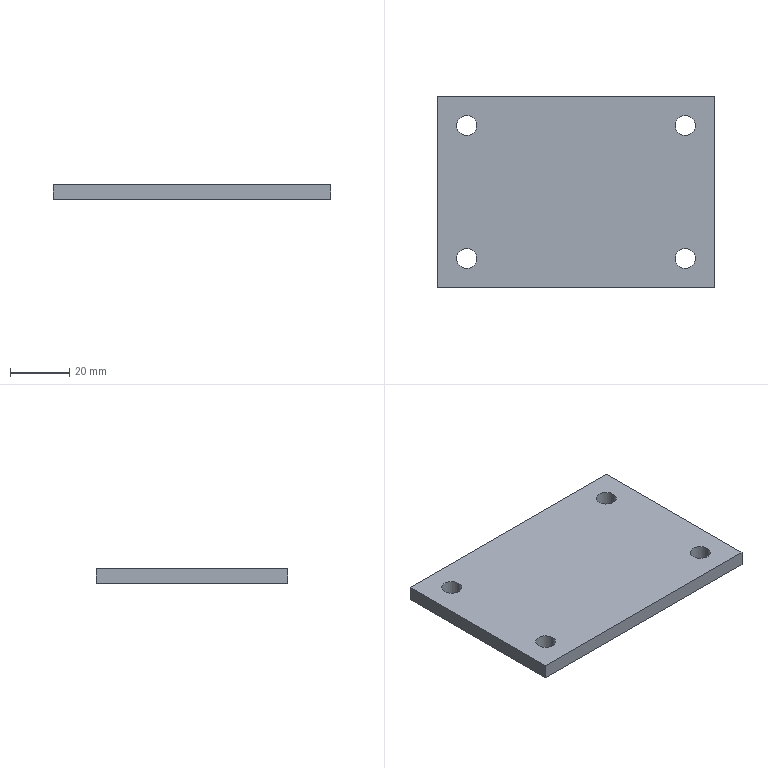Part | SolidWorks | features FlatPattern 1, SMBaseFlange 1, SheetMetal 1 | 1 solid | 14 faces | box 94 x 65 x 5 mm | volume 29824 mm3 | cylinder 8 | plane 6 | commonest cylinder face diameters 6.8 x8
STEP:
#1=CARTESIAN_POINT('',(-40.4,22.5,-5.));
#2=VERTEX_POINT('',#1);
#3=CARTESIAN_POINT('',(-33.6,22.5,-5.));
#4=VERTEX_POINT('',#3);
#5=CARTESIAN_POINT('',(-37.,22.5,-5.));
#6=DIRECTION('',(0.,0.,1.));
#7=DIRECTION('',(-1.,0.,0.));
#8=AXIS2_PLACEMENT_3D('',#5,#6,#7);
#9=CIRCLE('',#8,3.4);
#10=EDGE_CURVE('',#2,#4,#9,.T.);
#11=ORIENTED_EDGE('',*,*,#10,.F.);
#12=CARTESIAN_POINT('',(-40.4,22.5,0.));
#13=VERTEX_POINT('',#12);
#14=CARTESIAN_POINT('',(-40.4,22.5,-5.));
#15=DIRECTION('',(0.,0.,1.));
#16=VECTOR('',#15,1000.);
#17=LINE('',#14,#16);
#18=EDGE_CURVE('',#2,#13,#17,.T.);
#19=ORIENTED_EDGE('',*,*,#18,.T.);
#20=CARTESIAN_POINT('',(-33.6,22.5,0.));
#21=VERTEX_POINT('',#20);
#22=CARTESIAN_POINT('',(-37.,22.5,0.));
#23=DIRECTION('',(0.,0.,1.));
#24=DIRECTION('',(-1.,0.,0.));
#25=AXIS2_PLACEMENT_3D('',#22,#23,#24);
#26=CIRCLE('',#25,3.4);
#27=EDGE_CURVE('',#13,#21,#26,.T.);
#28=ORIENTED_EDGE('',*,*,#27,.T.);
#29=CARTESIAN_POINT('',(-33.6,22.5,-5.));
#30=DIRECTION('',(0.,0.,1.));
#31=VECTOR('',#30,1000.);
#32=LINE('',#29,#31);
#33=EDGE_CURVE('',#4,#21,#32,.T.);
#34=ORIENTED_EDGE('',*,*,#33,.F.);
#35=EDGE_LOOP('',(#11,#19,#28,#34));
#36=FACE_OUTER_BOUND('',#35,.T.);
#37=CARTESIAN_POINT('',(-37.,22.5,-5.));
#38=DIRECTION('',(0.,0.,1.));
#39=DIRECTION('',(1.,0.,0.));
#40=AXIS2_PLACEMENT_3D('',#37,#38,#39);
#41=CYLINDRICAL_SURFACE('',#40,3.4);
#42=ADVANCED_FACE('',(#36),#41,.F.);
#43=CARTESIAN_POINT('',(33.6,22.5,-5.));
#44=VERTEX_POINT('',#43);
#45=CARTESIAN_POINT('',(40.4,22.5,-5.));
#46=VERTEX_POINT('',#45);
#47=CARTESIAN_POINT('',(37.,22.5,-5.));
#48=DIRECTION('',(0.,0.,1.));
#49=DIRECTION('',(-1.,0.,0.));
#50=AXIS2_PLACEMENT_3D('',#47,#48,#49);
#51=CIRCLE('',#50,3.4);
#52=EDGE_CURVE('',#44,#46,#51,.T.);
#53=ORIENTED_EDGE('',*,*,#52,.F.);
#54=CARTESIAN_POINT('',(33.6,22.5,0.));
#55=VERTEX_POINT('',#54);
#56=CARTESIAN_POINT('',(33.6,22.5,-5.));
#57=DIRECTION('',(0.,0.,1.));
#58=VECTOR('',#57,1000.);
#59=LINE('',#56,#58);
#60=EDGE_CURVE('',#44,#55,#59,.T.);
#61=ORIENTED_EDGE('',*,*,#60,.T.);
#62=CARTESIAN_POINT('',(40.4,22.5,0.));
#63=VERTEX_POINT('',#62);
#64=CARTESIAN_POINT('',(37.,22.5,0.));
#65=DIRECTION('',(0.,0.,1.));
#66=DIRECTION('',(-1.,0.,0.));
#67=AXIS2_PLACEMENT_3D('',#64,#65,#66);
#68=CIRCLE('',#67,3.4);
#69=EDGE_CURVE('',#55,#63,#68,.T.);
#70=ORIENTED_EDGE('',*,*,#69,.T.);
#71=CARTESIAN_POINT('',(40.4,22.5,-5.));
#72=DIRECTION('',(0.,0.,1.));
#73=VECTOR('',#72,1000.);
#74=LINE('',#71,#73);
#75=EDGE_CURVE('',#46,#63,#74,.T.);
#76=ORIENTED_EDGE('',*,*,#75,.F.);
#77=EDGE_LOOP('',(#53,#61,#70,#76));
#78=FACE_OUTER_BOUND('',#77,.T.);
#79=CARTESIAN_POINT('',(37.,22.5,-5.));
#80=DIRECTION('',(0.,0.,1.));
#81=DIRECTION('',(1.,0.,0.));
#82=AXIS2_PLACEMENT_3D('',#79,#80,#81);
#83=CYLINDRICAL_SURFACE('',#82,3.4);
#84=ADVANCED_FACE('',(#78),#83,.F.);
#85=CARTESIAN_POINT('',(33.6,-22.5,-5.));
#86=VERTEX_POINT('',#85);
#87=CARTESIAN_POINT('',(40.4,-22.5,-5.));
#88=VERTEX_POINT('',#87);
#89=CARTESIAN_POINT('',(37.,-22.5,-5.));
#90=DIRECTION('',(0.,0.,1.));
#91=DIRECTION('',(1.,0.,0.));
#92=AXIS2_PLACEMENT_3D('',#89,#90,#91);
#93=CIRCLE('',#92,3.4);
#94=EDGE_CURVE('',#86,#88,#93,.T.);
#95=ORIENTED_EDGE('',*,*,#94,.F.);
#96=CARTESIAN_POINT('',(33.6,-22.5,0.));
#97=VERTEX_POINT('',#96);
#98=CARTESIAN_POINT('',(33.6,-22.5,-5.));
#99=DIRECTION('',(0.,0.,1.));
#100=VECTOR('',#99,1000.);
#101=LINE('',#98,#100);
#102=EDGE_CURVE('',#86,#97,#101,.T.);
#103=ORIENTED_EDGE('',*,*,#102,.T.);
#104=CARTESIAN_POINT('',(40.4,-22.5,0.));
#105=VERTEX_POINT('',#104);
#106=CARTESIAN_POINT('',(37.,-22.5,0.));
#107=DIRECTION('',(0.,0.,1.));
#108=DIRECTION('',(1.,0.,0.));
#109=AXIS2_PLACEMENT_3D('',#106,#107,#108);
#110=CIRCLE('',#109,3.4);
#111=EDGE_CURVE('',#97,#105,#110,.T.);
#112=ORIENTED_EDGE('',*,*,#111,.T.);
#113=CARTESIAN_POINT('',(40.4,-22.5,-5.));
#114=DIRECTION('',(0.,0.,1.));
#115=VECTOR('',#114,1000.);
#116=LINE('',#113,#115);
#117=EDGE_CURVE('',#88,#105,#116,.T.);
#118=ORIENTED_EDGE('',*,*,#117,.F.);
#119=EDGE_LOOP('',(#95,#103,#112,#118));
#120=FACE_OUTER_BOUND('',#119,.T.);
#121=CARTESIAN_POINT('',(37.,-22.5,-5.));
#122=DIRECTION('',(0.,0.,1.));
#123=DIRECTION('',(1.,0.,0.));
#124=AXIS2_PLACEMENT_3D('',#121,#122,#123);
#125=CYLINDRICAL_SURFACE('',#124,3.4);
#126=ADVANCED_FACE('',(#120),#125,.F.);
#127=CARTESIAN_POINT('',(-40.4,-22.5,-5.));
#128=VERTEX_POINT('',#127);
#129=CARTESIAN_POINT('',(-33.6,-22.5,-5.));
#130=VERTEX_POINT('',#129);
#131=CARTESIAN_POINT('',(-37.,-22.5,-5.));
#132=DIRECTION('',(0.,0.,1.));
#133=DIRECTION('',(1.,0.,0.));
#134=AXIS2_PLACEMENT_3D('',#131,#132,#133);
#135=CIRCLE('',#134,3.4);
#136=EDGE_CURVE('',#128,#130,#135,.T.);
#137=ORIENTED_EDGE('',*,*,#136,.F.);
#138=CARTESIAN_POINT('',(-40.4,-22.5,0.));
#139=VERTEX_POINT('',#138);
#140=CARTESIAN_POINT('',(-40.4,-22.5,-5.));
#141=DIRECTION('',(0.,0.,1.));
#142=VECTOR('',#141,1000.);
#143=LINE('',#140,#142);
#144=EDGE_CURVE('',#128,#139,#143,.T.);
#145=ORIENTED_EDGE('',*,*,#144,.T.);
#146=CARTESIAN_POINT('',(-33.6,-22.5,0.));
#147=VERTEX_POINT('',#146);
#148=CARTESIAN_POINT('',(-37.,-22.5,0.));
#149=DIRECTION('',(0.,0.,1.));
#150=DIRECTION('',(1.,0.,0.));
#151=AXIS2_PLACEMENT_3D('',#148,#149,#150);
#152=CIRCLE('',#151,3.4);
#153=EDGE_CURVE('',#139,#147,#152,.T.);
#154=ORIENTED_EDGE('',*,*,#153,.T.);
#155=CARTESIAN_POINT('',(-33.6,-22.5,-5.));
#156=DIRECTION('',(0.,0.,1.));
#157=VECTOR('',#156,1000.);
#158=LINE('',#155,#157);
#159=EDGE_CURVE('',#130,#147,#158,.T.);
#160=ORIENTED_EDGE('',*,*,#159,.F.);
#161=EDGE_LOOP('',(#137,#145,#154,#160));
#162=FACE_OUTER_BOUND('',#161,.T.);
#163=CARTESIAN_POINT('',(-37.,-22.5,-5.));
#164=DIRECTION('',(0.,0.,1.));
#165=DIRECTION('',(1.,0.,0.));
#166=AXIS2_PLACEMENT_3D('',#163,#164,#165);
#167=CYLINDRICAL_SURFACE('',#166,3.4);
#168=ADVANCED_FACE('',(#162),#167,.F.);
#169=CARTESIAN_POINT('',(-47.,32.5,0.));
#170=VERTEX_POINT('',#169);
#171=CARTESIAN_POINT('',(-47.,-32.5,0.));
#172=VERTEX_POINT('',#171);
#173=CARTESIAN_POINT('',(-47.,32.5,0.));
#174=DIRECTION('',(0.,-1.,0.));
#175=VECTOR('',#174,1000.);
#176=LINE('',#173,#175);
#177=EDGE_CURVE('',#170,#172,#176,.T.);
#178=ORIENTED_EDGE('',*,*,#177,.F.);
#179=CARTESIAN_POINT('',(-47.,32.5,-5.));
#180=VERTEX_POINT('',#179);
#181=CARTESIAN_POINT('',(-47.,32.5,-5.));
#182=DIRECTION('',(0.,0.,1.));
#183=VECTOR('',#182,1000.);
#184=LINE('',#181,#183);
#185=EDGE_CURVE('',#180,#170,#184,.T.);
#186=ORIENTED_EDGE('',*,*,#185,.F.);
#187=CARTESIAN_POINT('',(-47.,-32.5,-5.));
#188=VERTEX_POINT('',#187);
#189=CARTESIAN_POINT('',(-47.,32.5,-5.));
#190=DIRECTION('',(0.,-1.,0.));
#191=VECTOR('',#190,1000.);
#192=LINE('',#189,#191);
#193=EDGE_CURVE('',#180,#188,#192,.T.);
#194=ORIENTED_EDGE('',*,*,#193,.T.);
#195=CARTESIAN_POINT('',(-47.,-32.5,-5.));
#196=DIRECTION('',(0.,0.,1.));
#197=VECTOR('',#196,1000.);
#198=LINE('',#195,#197);
#199=EDGE_CURVE('',#188,#172,#198,.T.);
#200=ORIENTED_EDGE('',*,*,#199,.T.);
#201=EDGE_LOOP('',(#178,#186,#194,#200));
#202=FACE_OUTER_BOUND('',#201,.T.);
#203=CARTESIAN_POINT('',(-47.,32.5,-5.));
#204=DIRECTION('',(-1.,0.,0.));
#205=DIRECTION('',(0.,-1.,0.));
#206=AXIS2_PLACEMENT_3D('',#203,#204,#205);
#207=PLANE('',#206);
#208=ADVANCED_FACE('',(#202),#207,.T.);
#209=CARTESIAN_POINT('',(47.,32.5,0.));
#210=VERTEX_POINT('',#209);
#211=CARTESIAN_POINT('',(-47.,32.5,0.));
#212=DIRECTION('',(-1.,0.,0.));
#213=VECTOR('',#212,1000.);
#214=LINE('',#211,#213);
#215=EDGE_CURVE('',#210,#170,#214,.T.);
#216=ORIENTED_EDGE('',*,*,#215,.F.);
#217=CARTESIAN_POINT('',(47.,32.5,-5.));
#218=VERTEX_POINT('',#217);
#219=CARTESIAN_POINT('',(47.,32.5,-5.));
#220=DIRECTION('',(0.,0.,1.));
#221=VECTOR('',#220,1000.);
#222=LINE('',#219,#221);
#223=EDGE_CURVE('',#218,#210,#222,.T.);
#224=ORIENTED_EDGE('',*,*,#223,.F.);
#225=CARTESIAN_POINT('',(-47.,32.5,-5.));
#226=DIRECTION('',(-1.,0.,0.));
#227=VECTOR('',#226,1000.);
#228=LINE('',#225,#227);
#229=EDGE_CURVE('',#218,#180,#228,.T.);
#230=ORIENTED_EDGE('',*,*,#229,.T.);
#231=ORIENTED_EDGE('',*,*,#185,.T.);
#232=EDGE_LOOP('',(#216,#224,#230,#231));
#233=FACE_OUTER_BOUND('',#232,.T.);
#234=CARTESIAN_POINT('',(-47.,32.5,-5.));
#235=DIRECTION('',(0.,1.,0.));
#236=DIRECTION('',(-1.,0.,0.));
#237=AXIS2_PLACEMENT_3D('',#234,#235,#236);
#238=PLANE('',#237);
#239=ADVANCED_FACE('',(#233),#238,.T.);
#240=CARTESIAN_POINT('',(47.,-32.5,0.));
#241=VERTEX_POINT('',#240);
#242=CARTESIAN_POINT('',(47.,32.5,0.));
#243=DIRECTION('',(0.,1.,0.));
#244=VECTOR('',#243,1000.);
#245=LINE('',#242,#244);
#246=EDGE_CURVE('',#241,#210,#245,.T.);
#247=ORIENTED_EDGE('',*,*,#246,.F.);
#248=CARTESIAN_POINT('',(47.,-32.5,-5.));
#249=VERTEX_POINT('',#248);
#250=CARTESIAN_POINT('',(47.,-32.5,-5.));
#251=DIRECTION('',(0.,0.,1.));
#252=VECTOR('',#251,1000.);
#253=LINE('',#250,#252);
#254=EDGE_CURVE('',#249,#241,#253,.T.);
#255=ORIENTED_EDGE('',*,*,#254,.F.);
#256=CARTESIAN_POINT('',(47.,32.5,-5.));
#257=DIRECTION('',(0.,1.,0.));
#258=VECTOR('',#257,1000.);
#259=LINE('',#256,#258);
#260=EDGE_CURVE('',#249,#218,#259,.T.);
#261=ORIENTED_EDGE('',*,*,#260,.T.);
#262=ORIENTED_EDGE('',*,*,#223,.T.);
#263=EDGE_LOOP('',(#247,#255,#261,#262));
#264=FACE_OUTER_BOUND('',#263,.T.);
#265=CARTESIAN_POINT('',(47.,32.5,-5.));
#266=DIRECTION('',(1.,0.,0.));
#267=DIRECTION('',(0.,0.,-1.));
#268=AXIS2_PLACEMENT_3D('',#265,#266,#267);
#269=PLANE('',#268);
#270=ADVANCED_FACE('',(#264),#269,.T.);
#271=CARTESIAN_POINT('',(-47.,-32.5,0.));
#272=DIRECTION('',(1.,0.,0.));
#273=VECTOR('',#272,1000.);
#274=LINE('',#271,#273);
#275=EDGE_CURVE('',#172,#241,#274,.T.);
#276=ORIENTED_EDGE('',*,*,#275,.F.);
#277=ORIENTED_EDGE('',*,*,#199,.F.);
#278=CARTESIAN_POINT('',(-47.,-32.5,-5.));
#279=DIRECTION('',(1.,0.,0.));
#280=VECTOR('',#279,1000.);
#281=LINE('',#278,#280);
#282=EDGE_CURVE('',#188,#249,#281,.T.);
#283=ORIENTED_EDGE('',*,*,#282,.T.);
#284=ORIENTED_EDGE('',*,*,#254,.T.);
#285=EDGE_LOOP('',(#276,#277,#283,#284));
#286=FACE_OUTER_BOUND('',#285,.T.);
#287=CARTESIAN_POINT('',(-47.,-32.5,-5.));
#288=DIRECTION('',(0.,-1.,0.));
#289=DIRECTION('',(1.,0.,0.));
#290=AXIS2_PLACEMENT_3D('',#287,#288,#289);
#291=PLANE('',#290);
#292=ADVANCED_FACE('',(#286),#291,.T.);
#293=CARTESIAN_POINT('',(-37.,22.5,-5.));
#294=DIRECTION('',(0.,0.,1.));
#295=DIRECTION('',(-1.,0.,0.));
#296=AXIS2_PLACEMENT_3D('',#293,#294,#295);
#297=CIRCLE('',#296,3.4);
#298=EDGE_CURVE('',#4,#2,#297,.T.);
#299=ORIENTED_EDGE('',*,*,#298,.T.);
#300=ORIENTED_EDGE('',*,*,#10,.T.);
#301=EDGE_LOOP('',(#299,#300));
#302=FACE_BOUND('',#301,.T.);
#303=CARTESIAN_POINT('',(37.,22.5,-5.));
#304=DIRECTION('',(0.,0.,1.));
#305=DIRECTION('',(-1.,0.,0.));
#306=AXIS2_PLACEMENT_3D('',#303,#304,#305);
#307=CIRCLE('',#306,3.4);
#308=EDGE_CURVE('',#46,#44,#307,.T.);
#309=ORIENTED_EDGE('',*,*,#308,.T.);
#310=ORIENTED_EDGE('',*,*,#52,.T.);
#311=EDGE_LOOP('',(#309,#310));
#312=FACE_BOUND('',#311,.T.);
#313=CARTESIAN_POINT('',(37.,-22.5,-5.));
#314=DIRECTION('',(0.,0.,1.));
#315=DIRECTION('',(1.,0.,0.));
#316=AXIS2_PLACEMENT_3D('',#313,#314,#315);
#317=CIRCLE('',#316,3.4);
#318=EDGE_CURVE('',#88,#86,#317,.T.);
#319=ORIENTED_EDGE('',*,*,#318,.T.);
#320=ORIENTED_EDGE('',*,*,#94,.T.);
#321=EDGE_LOOP('',(#319,#320));
#322=FACE_BOUND('',#321,.T.);
#323=CARTESIAN_POINT('',(-37.,-22.5,-5.));
#324=DIRECTION('',(0.,0.,1.));
#325=DIRECTION('',(1.,0.,0.));
#326=AXIS2_PLACEMENT_3D('',#323,#324,#325);
#327=CIRCLE('',#326,3.4);
#328=EDGE_CURVE('',#130,#128,#327,.T.);
#329=ORIENTED_EDGE('',*,*,#328,.T.);
#330=ORIENTED_EDGE('',*,*,#136,.T.);
#331=EDGE_LOOP('',(#329,#330));
#332=FACE_BOUND('',#331,.T.);
#333=ORIENTED_EDGE('',*,*,#193,.F.);
#334=ORIENTED_EDGE('',*,*,#229,.F.);
#335=ORIENTED_EDGE('',*,*,#260,.F.);
#336=ORIENTED_EDGE('',*,*,#282,.F.);
#337=EDGE_LOOP('',(#333,#334,#335,#336));
#338=FACE_OUTER_BOUND('',#337,.T.);
#339=CARTESIAN_POINT('',(-47.,-32.5,-5.));
#340=DIRECTION('',(0.,0.,1.));
#341=DIRECTION('',(1.,0.,0.));
#342=AXIS2_PLACEMENT_3D('',#339,#340,#341);
#343=PLANE('',#342);
#344=ADVANCED_FACE('',(#302,#312,#322,#332,#338),#343,.F.);
#345=CARTESIAN_POINT('',(-37.,22.5,0.));
#346=DIRECTION('',(0.,0.,1.));
#347=DIRECTION('',(-1.,0.,0.));
#348=AXIS2_PLACEMENT_3D('',#345,#346,#347);
#349=CIRCLE('',#348,3.4);
#350=EDGE_CURVE('',#21,#13,#349,.T.);
#351=ORIENTED_EDGE('',*,*,#350,.F.);
#352=ORIENTED_EDGE('',*,*,#27,.F.);
#353=EDGE_LOOP('',(#351,#352));
#354=FACE_BOUND('',#353,.T.);
#355=CARTESIAN_POINT('',(37.,22.5,0.));
#356=DIRECTION('',(0.,0.,1.));
#357=DIRECTION('',(-1.,0.,0.));
#358=AXIS2_PLACEMENT_3D('',#355,#356,#357);
#359=CIRCLE('',#358,3.4);
#360=EDGE_CURVE('',#63,#55,#359,.T.);
#361=ORIENTED_EDGE('',*,*,#360,.F.);
#362=ORIENTED_EDGE('',*,*,#69,.F.);
#363=EDGE_LOOP('',(#361,#362));
#364=FACE_BOUND('',#363,.T.);
#365=CARTESIAN_POINT('',(37.,-22.5,0.));
#366=DIRECTION('',(0.,0.,1.));
#367=DIRECTION('',(1.,0.,0.));
#368=AXIS2_PLACEMENT_3D('',#365,#366,#367);
#369=CIRCLE('',#368,3.4);
#370=EDGE_CURVE('',#105,#97,#369,.T.);
#371=ORIENTED_EDGE('',*,*,#370,.F.);
#372=ORIENTED_EDGE('',*,*,#111,.F.);
#373=EDGE_LOOP('',(#371,#372));
#374=FACE_BOUND('',#373,.T.);
#375=CARTESIAN_POINT('',(-37.,-22.5,0.));
#376=DIRECTION('',(0.,0.,1.));
#377=DIRECTION('',(1.,0.,0.));
#378=AXIS2_PLACEMENT_3D('',#375,#376,#377);
#379=CIRCLE('',#378,3.4);
#380=EDGE_CURVE('',#147,#139,#379,.T.);
#381=ORIENTED_EDGE('',*,*,#380,.F.);
#382=ORIENTED_EDGE('',*,*,#153,.F.);
#383=EDGE_LOOP('',(#381,#382));
#384=FACE_BOUND('',#383,.T.);
#385=ORIENTED_EDGE('',*,*,#177,.T.);
#386=ORIENTED_EDGE('',*,*,#275,.T.);
#387=ORIENTED_EDGE('',*,*,#246,.T.);
#388=ORIENTED_EDGE('',*,*,#215,.T.);
#389=EDGE_LOOP('',(#385,#386,#387,#388));
#390=FACE_OUTER_BOUND('',#389,.T.);
#391=CARTESIAN_POINT('',(-47.,-32.5,0.));
#392=DIRECTION('',(0.,0.,1.));
#393=DIRECTION('',(1.,0.,0.));
#394=AXIS2_PLACEMENT_3D('',#391,#392,#393);
#395=PLANE('',#394);
#396=ADVANCED_FACE('',(#354,#364,#374,#384,#390),#395,.T.);
#397=ORIENTED_EDGE('',*,*,#144,.F.);
#398=ORIENTED_EDGE('',*,*,#328,.F.);
#399=ORIENTED_EDGE('',*,*,#159,.T.);
#400=ORIENTED_EDGE('',*,*,#380,.T.);
#401=EDGE_LOOP('',(#397,#398,#399,#400));
#402=FACE_OUTER_BOUND('',#401,.T.);
#403=CARTESIAN_POINT('',(-37.,-22.5,-5.));
#404=DIRECTION('',(0.,0.,1.));
#405=DIRECTION('',(1.,0.,0.));
#406=AXIS2_PLACEMENT_3D('',#403,#404,#405);
#407=CYLINDRICAL_SURFACE('',#406,3.4);
#408=ADVANCED_FACE('',(#402),#407,.F.);
#409=ORIENTED_EDGE('',*,*,#102,.F.);
#410=ORIENTED_EDGE('',*,*,#318,.F.);
#411=ORIENTED_EDGE('',*,*,#117,.T.);
#412=ORIENTED_EDGE('',*,*,#370,.T.);
#413=EDGE_LOOP('',(#409,#410,#411,#412));
#414=FACE_OUTER_BOUND('',#413,.T.);
#415=CARTESIAN_POINT('',(37.,-22.5,-5.));
#416=DIRECTION('',(0.,0.,1.));
#417=DIRECTION('',(1.,0.,0.));
#418=AXIS2_PLACEMENT_3D('',#415,#416,#417);
#419=CYLINDRICAL_SURFACE('',#418,3.4);
#420=ADVANCED_FACE('',(#414),#419,.F.);
#421=ORIENTED_EDGE('',*,*,#60,.F.);
#422=ORIENTED_EDGE('',*,*,#308,.F.);
#423=ORIENTED_EDGE('',*,*,#75,.T.);
#424=ORIENTED_EDGE('',*,*,#360,.T.);
#425=EDGE_LOOP('',(#421,#422,#423,#424));
#426=FACE_OUTER_BOUND('',#425,.T.);
#427=CARTESIAN_POINT('',(37.,22.5,-5.));
#428=DIRECTION('',(0.,0.,1.));
#429=DIRECTION('',(1.,0.,0.));
#430=AXIS2_PLACEMENT_3D('',#427,#428,#429);
#431=CYLINDRICAL_SURFACE('',#430,3.4);
#432=ADVANCED_FACE('',(#426),#431,.F.);
#433=ORIENTED_EDGE('',*,*,#18,.F.);
#434=ORIENTED_EDGE('',*,*,#298,.F.);
#435=ORIENTED_EDGE('',*,*,#33,.T.);
#436=ORIENTED_EDGE('',*,*,#350,.T.);
#437=EDGE_LOOP('',(#433,#434,#435,#436));
#438=FACE_OUTER_BOUND('',#437,.T.);
#439=CARTESIAN_POINT('',(-37.,22.5,-5.));
#440=DIRECTION('',(0.,0.,1.));
#441=DIRECTION('',(1.,0.,0.));
#442=AXIS2_PLACEMENT_3D('',#439,#440,#441);
#443=CYLINDRICAL_SURFACE('',#442,3.4);
#444=ADVANCED_FACE('',(#438),#443,.F.);
#445=CLOSED_SHELL('',(#42,#84,#126,#168,#208,#239,#270,#292,#344,#396,#408,#420,#432,#444));
#446=MANIFOLD_SOLID_BREP('',#445);
#447=CARTESIAN_POINT('',(0.,0.,0.));
#448=DIRECTION('',(0.,0.,1.));
#449=DIRECTION('',(1.,0.,0.));
#450=AXIS2_PLACEMENT_3D('',#447,#448,#449);
#451=(LENGTH_UNIT()NAMED_UNIT(*)SI_UNIT(.MILLI.,.METRE.));
#452=UNCERTAINTY_MEASURE_WITH_UNIT(LENGTH_MEASURE(0.00001),#451,'','');
#453=(NAMED_UNIT(*)PLANE_ANGLE_UNIT()SI_UNIT($,.RADIAN.));
#454=(NAMED_UNIT(*)SI_UNIT($,.STERADIAN.)SOLID_ANGLE_UNIT());
#455=(GEOMETRIC_REPRESENTATION_CONTEXT(3)GLOBAL_UNCERTAINTY_ASSIGNED_CONTEXT((#452))GLOBAL_UNIT_ASSIGNED_CONTEXT((#451,#453,#454))REPRESENTATION_CONTEXT('',''));
#456=ADVANCED_BREP_SHAPE_REPRESENTATION('',(#446,#450),#455);